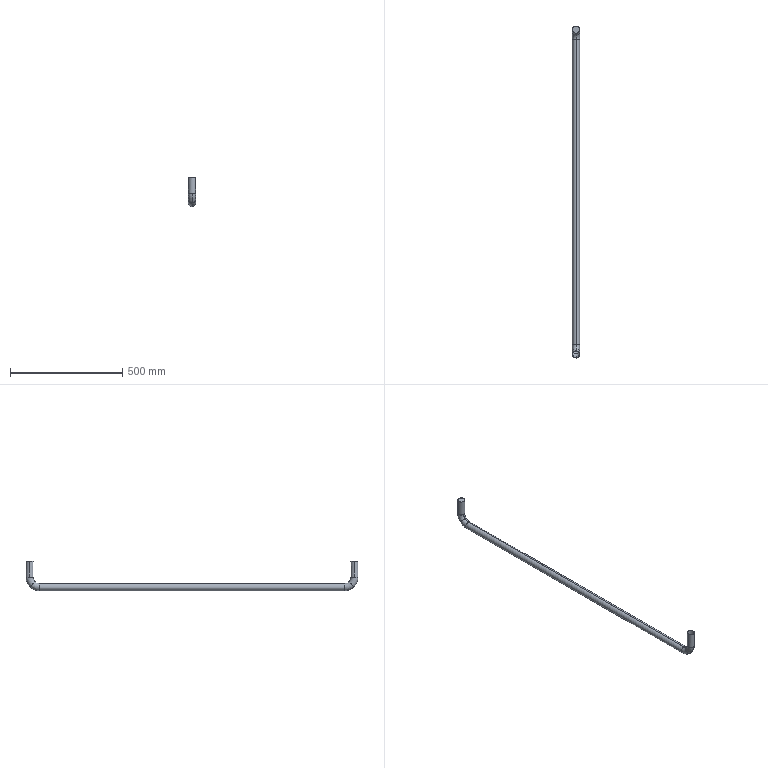Part | STEP file | 1 solid | 31 faces | box 32 x 1480 x 131 mm | volume 236738 mm3 | torus 16 | cylinder 12 | plane 3 | commonest cylinder face diameters 29 x6 32 x6